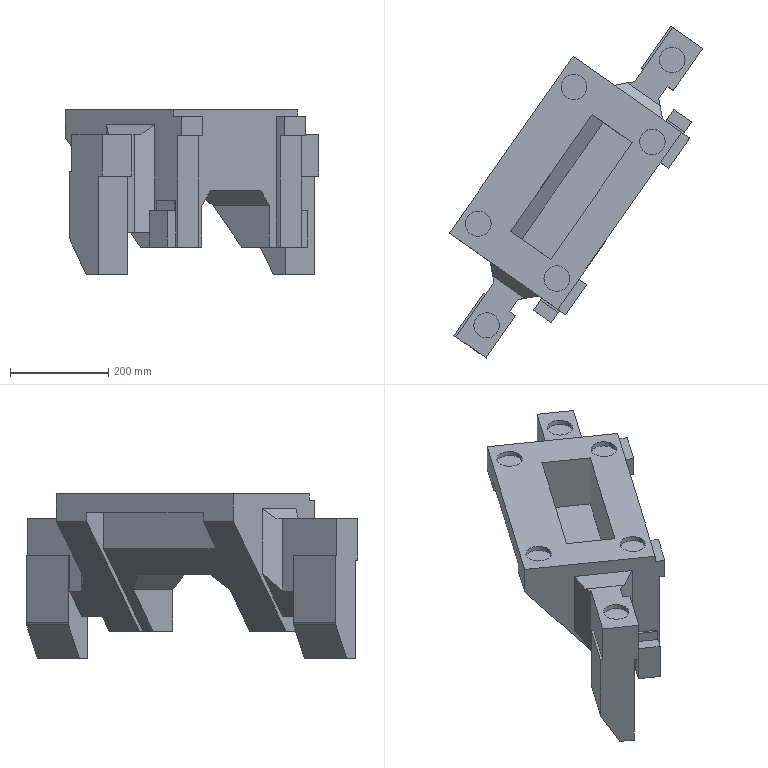Part | NX | features solid 2 | 1 solid | 99 faces | box 516.894 x 676.633 x 335 mm | volume 21948929 mm3 | plane 86 | cylinder 10 | spline 3 | commonest cylinder face diameters 52 x6 20 x2 58.2 x2